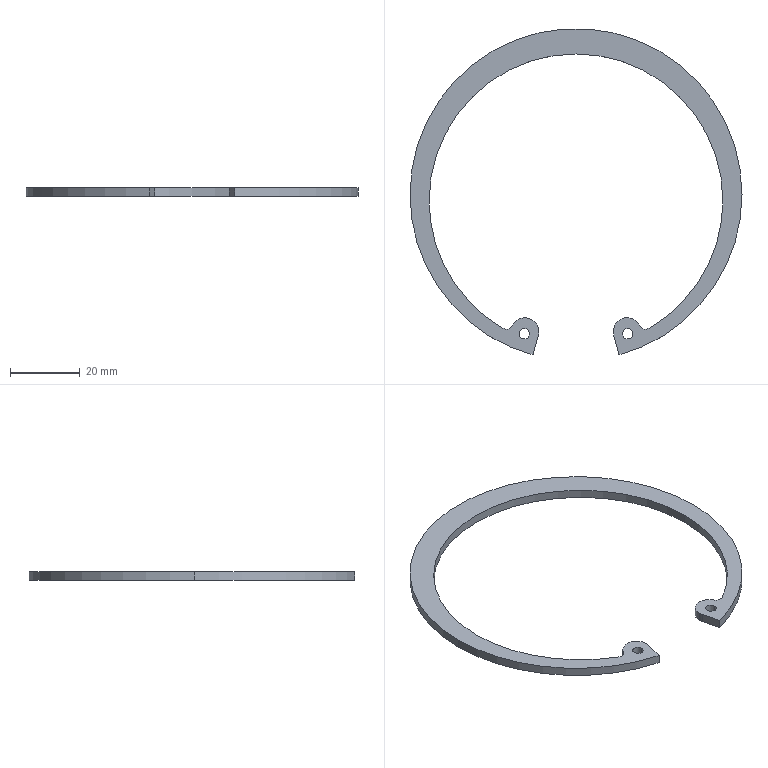Part | SolidWorks | features Extrusion 1 | 1 solid | 19 faces | box 95.5 x 93.873 x 2.5 mm | volume 3834 mm3 | cylinder 15 | plane 4 | commonest cylinder face diameters 3 x4 8 x3 84.5 x3 95.5 x3 4 x2
STEP:
#1=CARTESIAN_POINT('',(13.367,-40.028,1.25));
#2=VERTEX_POINT('',#1);
#3=CARTESIAN_POINT('',(16.367,-40.028,1.25));
#4=VERTEX_POINT('',#3);
#5=CARTESIAN_POINT('',(14.867,-40.028,1.25));
#6=DIRECTION('',(0.,0.,1.));
#7=DIRECTION('',(-1.,0.,0.));
#8=AXIS2_PLACEMENT_3D('',#5,#6,#7);
#9=CIRCLE('',#8,1.5);
#10=EDGE_CURVE('',#2,#4,#9,.T.);
#11=ORIENTED_EDGE('',*,*,#10,.T.);
#12=CARTESIAN_POINT('',(16.367,-40.028,-1.25));
#13=VERTEX_POINT('',#12);
#14=CARTESIAN_POINT('',(16.367,-40.028,1.25));
#15=DIRECTION('',(0.,0.,-1.));
#16=VECTOR('',#15,1000.);
#17=LINE('',#14,#16);
#18=EDGE_CURVE('',#4,#13,#17,.T.);
#19=ORIENTED_EDGE('',*,*,#18,.T.);
#20=CARTESIAN_POINT('',(13.367,-40.028,-1.25));
#21=VERTEX_POINT('',#20);
#22=CARTESIAN_POINT('',(14.867,-40.028,-1.25));
#23=DIRECTION('',(0.,0.,1.));
#24=DIRECTION('',(-1.,0.,0.));
#25=AXIS2_PLACEMENT_3D('',#22,#23,#24);
#26=CIRCLE('',#25,1.5);
#27=EDGE_CURVE('',#21,#13,#26,.T.);
#28=ORIENTED_EDGE('',*,*,#27,.F.);
#29=CARTESIAN_POINT('',(13.367,-40.028,1.25));
#30=DIRECTION('',(0.,0.,-1.));
#31=VECTOR('',#30,1000.);
#32=LINE('',#29,#31);
#33=EDGE_CURVE('',#2,#21,#32,.T.);
#34=ORIENTED_EDGE('',*,*,#33,.F.);
#35=EDGE_LOOP('',(#11,#19,#28,#34));
#36=FACE_OUTER_BOUND('',#35,.T.);
#37=CARTESIAN_POINT('',(14.867,-40.028,1.25));
#38=DIRECTION('',(0.,0.,-1.));
#39=DIRECTION('',(-1.,0.,0.));
#40=AXIS2_PLACEMENT_3D('',#37,#38,#39);
#41=CYLINDRICAL_SURFACE('',#40,1.5);
#42=ADVANCED_FACE('',(#36),#41,.F.);
#43=CARTESIAN_POINT('',(-16.367,-40.028,1.25));
#44=VERTEX_POINT('',#43);
#45=CARTESIAN_POINT('',(-13.367,-40.028,1.25));
#46=VERTEX_POINT('',#45);
#47=CARTESIAN_POINT('',(-14.867,-40.028,1.25));
#48=DIRECTION('',(0.,0.,1.));
#49=DIRECTION('',(1.,0.,0.));
#50=AXIS2_PLACEMENT_3D('',#47,#48,#49);
#51=CIRCLE('',#50,1.5);
#52=EDGE_CURVE('',#44,#46,#51,.T.);
#53=ORIENTED_EDGE('',*,*,#52,.T.);
#54=CARTESIAN_POINT('',(-13.367,-40.028,-1.25));
#55=VERTEX_POINT('',#54);
#56=CARTESIAN_POINT('',(-13.367,-40.028,1.25));
#57=DIRECTION('',(0.,0.,-1.));
#58=VECTOR('',#57,1000.);
#59=LINE('',#56,#58);
#60=EDGE_CURVE('',#46,#55,#59,.T.);
#61=ORIENTED_EDGE('',*,*,#60,.T.);
#62=CARTESIAN_POINT('',(-16.367,-40.028,-1.25));
#63=VERTEX_POINT('',#62);
#64=CARTESIAN_POINT('',(-14.867,-40.028,-1.25));
#65=DIRECTION('',(0.,0.,1.));
#66=DIRECTION('',(1.,0.,0.));
#67=AXIS2_PLACEMENT_3D('',#64,#65,#66);
#68=CIRCLE('',#67,1.5);
#69=EDGE_CURVE('',#63,#55,#68,.T.);
#70=ORIENTED_EDGE('',*,*,#69,.F.);
#71=CARTESIAN_POINT('',(-16.367,-40.028,1.25));
#72=DIRECTION('',(0.,0.,-1.));
#73=VECTOR('',#72,1000.);
#74=LINE('',#71,#73);
#75=EDGE_CURVE('',#44,#63,#74,.T.);
#76=ORIENTED_EDGE('',*,*,#75,.F.);
#77=EDGE_LOOP('',(#53,#61,#70,#76));
#78=FACE_OUTER_BOUND('',#77,.T.);
#79=CARTESIAN_POINT('',(-14.867,-40.028,1.25));
#80=DIRECTION('',(0.,0.,-1.));
#81=DIRECTION('',(-1.,0.,0.));
#82=AXIS2_PLACEMENT_3D('',#79,#80,#81);
#83=CYLINDRICAL_SURFACE('',#82,1.5);
#84=ADVANCED_FACE('',(#78),#83,.F.);
#85=CARTESIAN_POINT('',(47.75,0.,1.25));
#86=VERTEX_POINT('',#85);
#87=CARTESIAN_POINT('',(-47.75,0.,1.25));
#88=VERTEX_POINT('',#87);
#89=CARTESIAN_POINT('',(0.,0.,1.25));
#90=DIRECTION('',(0.,0.,1.));
#91=DIRECTION('',(1.,0.,0.));
#92=AXIS2_PLACEMENT_3D('',#89,#90,#91);
#93=CIRCLE('',#92,47.75);
#94=EDGE_CURVE('',#86,#88,#93,.T.);
#95=ORIENTED_EDGE('',*,*,#94,.F.);
#96=CARTESIAN_POINT('',(47.75,0.,-1.25));
#97=VERTEX_POINT('',#96);
#98=CARTESIAN_POINT('',(47.75,0.,1.25));
#99=DIRECTION('',(0.,0.,-1.));
#100=VECTOR('',#99,1000.);
#101=LINE('',#98,#100);
#102=EDGE_CURVE('',#86,#97,#101,.T.);
#103=ORIENTED_EDGE('',*,*,#102,.T.);
#104=CARTESIAN_POINT('',(-47.75,0.,-1.25));
#105=VERTEX_POINT('',#104);
#106=CARTESIAN_POINT('',(0.,0.,-1.25));
#107=DIRECTION('',(0.,0.,1.));
#108=DIRECTION('',(1.,0.,0.));
#109=AXIS2_PLACEMENT_3D('',#106,#107,#108);
#110=CIRCLE('',#109,47.75);
#111=EDGE_CURVE('',#97,#105,#110,.T.);
#112=ORIENTED_EDGE('',*,*,#111,.T.);
#113=CARTESIAN_POINT('',(-47.75,0.,1.25));
#114=DIRECTION('',(0.,0.,-1.));
#115=VECTOR('',#114,1000.);
#116=LINE('',#113,#115);
#117=EDGE_CURVE('',#88,#105,#116,.T.);
#118=ORIENTED_EDGE('',*,*,#117,.F.);
#119=EDGE_LOOP('',(#95,#103,#112,#118));
#120=FACE_OUTER_BOUND('',#119,.T.);
#121=CARTESIAN_POINT('',(0.,0.,1.25));
#122=DIRECTION('',(0.,0.,-1.));
#123=DIRECTION('',(-1.,0.,0.));
#124=AXIS2_PLACEMENT_3D('',#121,#122,#123);
#125=CYLINDRICAL_SURFACE('',#124,47.75);
#126=ADVANCED_FACE('',(#120),#125,.T.);
#127=CARTESIAN_POINT('',(-12.359,-46.123,1.25));
#128=VERTEX_POINT('',#127);
#129=CARTESIAN_POINT('',(0.,0.,1.25));
#130=DIRECTION('',(0.,0.,1.));
#131=DIRECTION('',(1.,0.,0.));
#132=AXIS2_PLACEMENT_3D('',#129,#130,#131);
#133=CIRCLE('',#132,47.75);
#134=EDGE_CURVE('',#88,#128,#133,.T.);
#135=ORIENTED_EDGE('',*,*,#134,.F.);
#136=ORIENTED_EDGE('',*,*,#117,.T.);
#137=CARTESIAN_POINT('',(-12.359,-46.123,-1.25));
#138=VERTEX_POINT('',#137);
#139=CARTESIAN_POINT('',(0.,0.,-1.25));
#140=DIRECTION('',(0.,0.,1.));
#141=DIRECTION('',(1.,0.,0.));
#142=AXIS2_PLACEMENT_3D('',#139,#140,#141);
#143=CIRCLE('',#142,47.75);
#144=EDGE_CURVE('',#105,#138,#143,.T.);
#145=ORIENTED_EDGE('',*,*,#144,.T.);
#146=CARTESIAN_POINT('',(-12.359,-46.123,1.25));
#147=DIRECTION('',(0.,0.,-1.));
#148=VECTOR('',#147,1000.);
#149=LINE('',#146,#148);
#150=EDGE_CURVE('',#128,#138,#149,.T.);
#151=ORIENTED_EDGE('',*,*,#150,.F.);
#152=EDGE_LOOP('',(#135,#136,#145,#151));
#153=FACE_OUTER_BOUND('',#152,.T.);
#154=CARTESIAN_POINT('',(0.,0.,1.25));
#155=DIRECTION('',(0.,0.,-1.));
#156=DIRECTION('',(-1.,0.,0.));
#157=AXIS2_PLACEMENT_3D('',#154,#155,#156);
#158=CYLINDRICAL_SURFACE('',#157,47.75);
#159=ADVANCED_FACE('',(#153),#158,.T.);
#160=CARTESIAN_POINT('',(10.698,-39.398,1.25));
#161=VERTEX_POINT('',#160);
#162=CARTESIAN_POINT('',(10.834,-40.433,1.25));
#163=VERTEX_POINT('',#162);
#164=CARTESIAN_POINT('',(14.698,-39.398,1.25));
#165=DIRECTION('',(0.,0.,1.));
#166=DIRECTION('',(-1.,0.,0.));
#167=AXIS2_PLACEMENT_3D('',#164,#165,#166);
#168=CIRCLE('',#167,4.);
#169=EDGE_CURVE('',#161,#163,#168,.T.);
#170=ORIENTED_EDGE('',*,*,#169,.F.);
#171=CARTESIAN_POINT('',(10.698,-39.398,-1.25));
#172=VERTEX_POINT('',#171);
#173=CARTESIAN_POINT('',(10.698,-39.398,1.25));
#174=DIRECTION('',(0.,0.,-1.));
#175=VECTOR('',#174,1000.);
#176=LINE('',#173,#175);
#177=EDGE_CURVE('',#161,#172,#176,.T.);
#178=ORIENTED_EDGE('',*,*,#177,.T.);
#179=CARTESIAN_POINT('',(10.834,-40.433,-1.25));
#180=VERTEX_POINT('',#179);
#181=CARTESIAN_POINT('',(14.698,-39.398,-1.25));
#182=DIRECTION('',(0.,0.,1.));
#183=DIRECTION('',(-1.,0.,0.));
#184=AXIS2_PLACEMENT_3D('',#181,#182,#183);
#185=CIRCLE('',#184,4.);
#186=EDGE_CURVE('',#172,#180,#185,.T.);
#187=ORIENTED_EDGE('',*,*,#186,.T.);
#188=CARTESIAN_POINT('',(10.834,-40.433,1.25));
#189=DIRECTION('',(0.,0.,-1.));
#190=VECTOR('',#189,1000.);
#191=LINE('',#188,#190);
#192=EDGE_CURVE('',#163,#180,#191,.T.);
#193=ORIENTED_EDGE('',*,*,#192,.F.);
#194=EDGE_LOOP('',(#170,#178,#187,#193));
#195=FACE_OUTER_BOUND('',#194,.T.);
#196=CARTESIAN_POINT('',(14.698,-39.398,1.25));
#197=DIRECTION('',(0.,0.,-1.));
#198=DIRECTION('',(-1.,0.,0.));
#199=AXIS2_PLACEMENT_3D('',#196,#197,#198);
#200=CYLINDRICAL_SURFACE('',#199,4.);
#201=ADVANCED_FACE('',(#195),#200,.T.);
#202=CARTESIAN_POINT('',(42.25,-1.8,1.25));
#203=VERTEX_POINT('',#202);
#204=CARTESIAN_POINT('',(21.052,-38.431,1.25));
#205=VERTEX_POINT('',#204);
#206=CARTESIAN_POINT('',(0.,-1.8,1.25));
#207=DIRECTION('',(0.,0.,-1.));
#208=DIRECTION('',(1.,0.,0.));
#209=AXIS2_PLACEMENT_3D('',#206,#207,#208);
#210=CIRCLE('',#209,42.25);
#211=EDGE_CURVE('',#203,#205,#210,.T.);
#212=ORIENTED_EDGE('',*,*,#211,.F.);
#213=CARTESIAN_POINT('',(42.25,-1.8,-1.25));
#214=VERTEX_POINT('',#213);
#215=CARTESIAN_POINT('',(42.25,-1.8,1.25));
#216=DIRECTION('',(0.,0.,-1.));
#217=VECTOR('',#216,1000.);
#218=LINE('',#215,#217);
#219=EDGE_CURVE('',#203,#214,#218,.T.);
#220=ORIENTED_EDGE('',*,*,#219,.T.);
#221=CARTESIAN_POINT('',(21.052,-38.431,-1.25));
#222=VERTEX_POINT('',#221);
#223=CARTESIAN_POINT('',(0.,-1.8,-1.25));
#224=DIRECTION('',(0.,0.,-1.));
#225=DIRECTION('',(1.,0.,0.));
#226=AXIS2_PLACEMENT_3D('',#223,#224,#225);
#227=CIRCLE('',#226,42.25);
#228=EDGE_CURVE('',#214,#222,#227,.T.);
#229=ORIENTED_EDGE('',*,*,#228,.T.);
#230=CARTESIAN_POINT('',(21.052,-38.431,1.25));
#231=DIRECTION('',(0.,0.,-1.));
#232=VECTOR('',#231,1000.);
#233=LINE('',#230,#232);
#234=EDGE_CURVE('',#205,#222,#233,.T.);
#235=ORIENTED_EDGE('',*,*,#234,.F.);
#236=EDGE_LOOP('',(#212,#220,#229,#235));
#237=FACE_OUTER_BOUND('',#236,.T.);
#238=CARTESIAN_POINT('',(0.,-1.8,1.25));
#239=DIRECTION('',(0.,0.,-1.));
#240=DIRECTION('',(-1.,0.,0.));
#241=AXIS2_PLACEMENT_3D('',#238,#239,#240);
#242=CYLINDRICAL_SURFACE('',#241,42.25);
#243=ADVANCED_FACE('',(#237),#242,.F.);
#244=ORIENTED_EDGE('',*,*,#219,.F.);
#245=CARTESIAN_POINT('',(-42.25,-1.8,1.25));
#246=VERTEX_POINT('',#245);
#247=CARTESIAN_POINT('',(0.,-1.8,1.25));
#248=DIRECTION('',(0.,0.,-1.));
#249=DIRECTION('',(1.,0.,0.));
#250=AXIS2_PLACEMENT_3D('',#247,#248,#249);
#251=CIRCLE('',#250,42.25);
#252=EDGE_CURVE('',#246,#203,#251,.T.);
#253=ORIENTED_EDGE('',*,*,#252,.F.);
#254=CARTESIAN_POINT('',(-42.25,-1.8,-1.25));
#255=VERTEX_POINT('',#254);
#256=CARTESIAN_POINT('',(-42.25,-1.8,1.25));
#257=DIRECTION('',(0.,0.,-1.));
#258=VECTOR('',#257,1000.);
#259=LINE('',#256,#258);
#260=EDGE_CURVE('',#246,#255,#259,.T.);
#261=ORIENTED_EDGE('',*,*,#260,.T.);
#262=CARTESIAN_POINT('',(0.,-1.8,-1.25));
#263=DIRECTION('',(0.,0.,-1.));
#264=DIRECTION('',(1.,0.,0.));
#265=AXIS2_PLACEMENT_3D('',#262,#263,#264);
#266=CIRCLE('',#265,42.25);
#267=EDGE_CURVE('',#255,#214,#266,.T.);
#268=ORIENTED_EDGE('',*,*,#267,.T.);
#269=EDGE_LOOP('',(#244,#253,#261,#268));
#270=FACE_OUTER_BOUND('',#269,.T.);
#271=CARTESIAN_POINT('',(0.,-1.8,1.25));
#272=DIRECTION('',(0.,0.,-1.));
#273=DIRECTION('',(-1.,0.,0.));
#274=AXIS2_PLACEMENT_3D('',#271,#272,#273);
#275=CYLINDRICAL_SURFACE('',#274,42.25);
#276=ADVANCED_FACE('',(#270),#275,.F.);
#277=ORIENTED_EDGE('',*,*,#52,.F.);
#278=CARTESIAN_POINT('',(-14.867,-40.028,1.25));
#279=DIRECTION('',(0.,0.,1.));
#280=DIRECTION('',(1.,0.,0.));
#281=AXIS2_PLACEMENT_3D('',#278,#279,#280);
#282=CIRCLE('',#281,1.5);
#283=EDGE_CURVE('',#46,#44,#282,.T.);
#284=ORIENTED_EDGE('',*,*,#283,.F.);
#285=EDGE_LOOP('',(#277,#284));
#286=FACE_BOUND('',#285,.T.);
#287=CARTESIAN_POINT('',(-10.834,-40.433,1.25));
#288=VERTEX_POINT('',#287);
#289=CARTESIAN_POINT('',(-18.27,-37.598,1.25));
#290=VERTEX_POINT('',#289);
#291=CARTESIAN_POINT('',(-14.698,-39.398,1.25));
#292=DIRECTION('',(0.,0.,1.));
#293=DIRECTION('',(1.,0.,0.));
#294=AXIS2_PLACEMENT_3D('',#291,#292,#293);
#295=CIRCLE('',#294,4.);
#296=EDGE_CURVE('',#288,#290,#295,.T.);
#297=ORIENTED_EDGE('',*,*,#296,.T.);
#298=CARTESIAN_POINT('',(-21.052,-38.431,1.25));
#299=VERTEX_POINT('',#298);
#300=CARTESIAN_POINT('',(-20.056,-36.697,1.25));
#301=DIRECTION('',(0.,0.,-1.));
#302=DIRECTION('',(-1.,0.,0.));
#303=AXIS2_PLACEMENT_3D('',#300,#301,#302);
#304=CIRCLE('',#303,2.);
#305=EDGE_CURVE('',#290,#299,#304,.T.);
#306=ORIENTED_EDGE('',*,*,#305,.T.);
#307=CARTESIAN_POINT('',(0.,-1.8,1.25));
#308=DIRECTION('',(0.,0.,-1.));
#309=DIRECTION('',(1.,0.,0.));
#310=AXIS2_PLACEMENT_3D('',#307,#308,#309);
#311=CIRCLE('',#310,42.25);
#312=EDGE_CURVE('',#299,#246,#311,.T.);
#313=ORIENTED_EDGE('',*,*,#312,.T.);
#314=ORIENTED_EDGE('',*,*,#252,.T.);
#315=ORIENTED_EDGE('',*,*,#211,.T.);
#316=CARTESIAN_POINT('',(18.27,-37.598,1.25));
#317=VERTEX_POINT('',#316);
#318=CARTESIAN_POINT('',(20.056,-36.697,1.25));
#319=DIRECTION('',(0.,0.,-1.));
#320=DIRECTION('',(1.,0.,0.));
#321=AXIS2_PLACEMENT_3D('',#318,#319,#320);
#322=CIRCLE('',#321,2.);
#323=EDGE_CURVE('',#205,#317,#322,.T.);
#324=ORIENTED_EDGE('',*,*,#323,.T.);
#325=CARTESIAN_POINT('',(14.698,-39.398,1.25));
#326=DIRECTION('',(0.,0.,1.));
#327=DIRECTION('',(-1.,0.,0.));
#328=AXIS2_PLACEMENT_3D('',#325,#326,#327);
#329=CIRCLE('',#328,4.);
#330=EDGE_CURVE('',#317,#161,#329,.T.);
#331=ORIENTED_EDGE('',*,*,#330,.T.);
#332=ORIENTED_EDGE('',*,*,#169,.T.);
#333=CARTESIAN_POINT('',(12.359,-46.123,1.25));
#334=VERTEX_POINT('',#333);
#335=CARTESIAN_POINT('',(10.834,-40.433,1.25));
#336=DIRECTION('',(0.2588,-0.9659,0.));
#337=VECTOR('',#336,1000.);
#338=LINE('',#335,#337);
#339=EDGE_CURVE('',#163,#334,#338,.T.);
#340=ORIENTED_EDGE('',*,*,#339,.T.);
#341=CARTESIAN_POINT('',(0.,0.,1.25));
#342=DIRECTION('',(0.,0.,1.));
#343=DIRECTION('',(1.,0.,0.));
#344=AXIS2_PLACEMENT_3D('',#341,#342,#343);
#345=CIRCLE('',#344,47.75);
#346=EDGE_CURVE('',#334,#86,#345,.T.);
#347=ORIENTED_EDGE('',*,*,#346,.T.);
#348=ORIENTED_EDGE('',*,*,#94,.T.);
#349=ORIENTED_EDGE('',*,*,#134,.T.);
#350=CARTESIAN_POINT('',(-10.834,-40.433,1.25));
#351=DIRECTION('',(0.2588,0.9659,0.));
#352=VECTOR('',#351,1000.);
#353=LINE('',#350,#352);
#354=EDGE_CURVE('',#128,#288,#353,.T.);
#355=ORIENTED_EDGE('',*,*,#354,.T.);
#356=EDGE_LOOP('',(#297,#306,#313,#314,#315,#324,#331,#332,#340,#347,#348,#349,#355));
#357=FACE_OUTER_BOUND('',#356,.T.);
#358=ORIENTED_EDGE('',*,*,#10,.F.);
#359=CARTESIAN_POINT('',(14.867,-40.028,1.25));
#360=DIRECTION('',(0.,0.,1.));
#361=DIRECTION('',(-1.,0.,0.));
#362=AXIS2_PLACEMENT_3D('',#359,#360,#361);
#363=CIRCLE('',#362,1.5);
#364=EDGE_CURVE('',#4,#2,#363,.T.);
#365=ORIENTED_EDGE('',*,*,#364,.F.);
#366=EDGE_LOOP('',(#358,#365));
#367=FACE_BOUND('',#366,.T.);
#368=CARTESIAN_POINT('',(-14.698,-39.398,1.25));
#369=DIRECTION('',(0.,0.,1.));
#370=DIRECTION('',(1.,0.,0.));
#371=AXIS2_PLACEMENT_3D('',#368,#369,#370);
#372=PLANE('',#371);
#373=ADVANCED_FACE('',(#286,#357,#367),#372,.T.);
#374=CARTESIAN_POINT('',(-10.834,-40.433,-1.25));
#375=VERTEX_POINT('',#374);
#376=CARTESIAN_POINT('',(-10.834,-40.433,1.25));
#377=DIRECTION('',(0.,0.,-1.));
#378=VECTOR('',#377,1000.);
#379=LINE('',#376,#378);
#380=EDGE_CURVE('',#288,#375,#379,.T.);
#381=ORIENTED_EDGE('',*,*,#380,.T.);
#382=CARTESIAN_POINT('',(-18.27,-37.598,-1.25));
#383=VERTEX_POINT('',#382);
#384=CARTESIAN_POINT('',(-14.698,-39.398,-1.25));
#385=DIRECTION('',(0.,0.,1.));
#386=DIRECTION('',(1.,0.,0.));
#387=AXIS2_PLACEMENT_3D('',#384,#385,#386);
#388=CIRCLE('',#387,4.);
#389=EDGE_CURVE('',#375,#383,#388,.T.);
#390=ORIENTED_EDGE('',*,*,#389,.T.);
#391=CARTESIAN_POINT('',(-18.27,-37.598,1.25));
#392=DIRECTION('',(0.,0.,-1.));
#393=VECTOR('',#392,1000.);
#394=LINE('',#391,#393);
#395=EDGE_CURVE('',#290,#383,#394,.T.);
#396=ORIENTED_EDGE('',*,*,#395,.F.);
#397=ORIENTED_EDGE('',*,*,#296,.F.);
#398=EDGE_LOOP('',(#381,#390,#396,#397));
#399=FACE_OUTER_BOUND('',#398,.T.);
#400=CARTESIAN_POINT('',(-14.698,-39.398,1.25));
#401=DIRECTION('',(0.,0.,-1.));
#402=DIRECTION('',(-1.,0.,0.));
#403=AXIS2_PLACEMENT_3D('',#400,#401,#402);
#404=CYLINDRICAL_SURFACE('',#403,4.);
#405=ADVANCED_FACE('',(#399),#404,.T.);
#406=ORIENTED_EDGE('',*,*,#395,.T.);
#407=CARTESIAN_POINT('',(-21.052,-38.431,-1.25));
#408=VERTEX_POINT('',#407);
#409=CARTESIAN_POINT('',(-20.056,-36.697,-1.25));
#410=DIRECTION('',(0.,0.,-1.));
#411=DIRECTION('',(-1.,0.,0.));
#412=AXIS2_PLACEMENT_3D('',#409,#410,#411);
#413=CIRCLE('',#412,2.);
#414=EDGE_CURVE('',#383,#408,#413,.T.);
#415=ORIENTED_EDGE('',*,*,#414,.T.);
#416=CARTESIAN_POINT('',(-21.052,-38.431,1.25));
#417=DIRECTION('',(0.,0.,-1.));
#418=VECTOR('',#417,1000.);
#419=LINE('',#416,#418);
#420=EDGE_CURVE('',#299,#408,#419,.T.);
#421=ORIENTED_EDGE('',*,*,#420,.F.);
#422=ORIENTED_EDGE('',*,*,#305,.F.);
#423=EDGE_LOOP('',(#406,#415,#421,#422));
#424=FACE_OUTER_BOUND('',#423,.T.);
#425=CARTESIAN_POINT('',(-20.056,-36.697,1.25));
#426=DIRECTION('',(0.,0.,-1.));
#427=DIRECTION('',(-1.,0.,0.));
#428=AXIS2_PLACEMENT_3D('',#425,#426,#427);
#429=CYLINDRICAL_SURFACE('',#428,2.);
#430=ADVANCED_FACE('',(#424),#429,.F.);
#431=ORIENTED_EDGE('',*,*,#260,.F.);
#432=ORIENTED_EDGE('',*,*,#312,.F.);
#433=ORIENTED_EDGE('',*,*,#420,.T.);
#434=CARTESIAN_POINT('',(0.,-1.8,-1.25));
#435=DIRECTION('',(0.,0.,-1.));
#436=DIRECTION('',(1.,0.,0.));
#437=AXIS2_PLACEMENT_3D('',#434,#435,#436);
#438=CIRCLE('',#437,42.25);
#439=EDGE_CURVE('',#408,#255,#438,.T.);
#440=ORIENTED_EDGE('',*,*,#439,.T.);
#441=EDGE_LOOP('',(#431,#432,#433,#440));
#442=FACE_OUTER_BOUND('',#441,.T.);
#443=CARTESIAN_POINT('',(0.,-1.8,1.25));
#444=DIRECTION('',(0.,0.,-1.));
#445=DIRECTION('',(-1.,0.,0.));
#446=AXIS2_PLACEMENT_3D('',#443,#444,#445);
#447=CYLINDRICAL_SURFACE('',#446,42.25);
#448=ADVANCED_FACE('',(#442),#447,.F.);
#449=ORIENTED_EDGE('',*,*,#234,.T.);
#450=CARTESIAN_POINT('',(18.27,-37.598,-1.25));
#451=VERTEX_POINT('',#450);
#452=CARTESIAN_POINT('',(20.056,-36.697,-1.25));
#453=DIRECTION('',(0.,0.,-1.));
#454=DIRECTION('',(1.,0.,0.));
#455=AXIS2_PLACEMENT_3D('',#452,#453,#454);
#456=CIRCLE('',#455,2.);
#457=EDGE_CURVE('',#222,#451,#456,.T.);
#458=ORIENTED_EDGE('',*,*,#457,.T.);
#459=CARTESIAN_POINT('',(18.27,-37.598,1.25));
#460=DIRECTION('',(0.,0.,-1.));
#461=VECTOR('',#460,1000.);
#462=LINE('',#459,#461);
#463=EDGE_CURVE('',#317,#451,#462,.T.);
#464=ORIENTED_EDGE('',*,*,#463,.F.);
#465=ORIENTED_EDGE('',*,*,#323,.F.);
#466=EDGE_LOOP('',(#449,#458,#464,#465));
#467=FACE_OUTER_BOUND('',#466,.T.);
#468=CARTESIAN_POINT('',(20.056,-36.697,1.25));
#469=DIRECTION('',(0.,0.,-1.));
#470=DIRECTION('',(-1.,0.,0.));
#471=AXIS2_PLACEMENT_3D('',#468,#469,#470);
#472=CYLINDRICAL_SURFACE('',#471,2.);
#473=ADVANCED_FACE('',(#467),#472,.F.);
#474=ORIENTED_EDGE('',*,*,#177,.F.);
#475=ORIENTED_EDGE('',*,*,#330,.F.);
#476=ORIENTED_EDGE('',*,*,#463,.T.);
#477=CARTESIAN_POINT('',(14.698,-39.398,-1.25));
#478=DIRECTION('',(0.,0.,1.));
#479=DIRECTION('',(-1.,0.,0.));
#480=AXIS2_PLACEMENT_3D('',#477,#478,#479);
#481=CIRCLE('',#480,4.);
#482=EDGE_CURVE('',#451,#172,#481,.T.);
#483=ORIENTED_EDGE('',*,*,#482,.T.);
#484=EDGE_LOOP('',(#474,#475,#476,#483));
#485=FACE_OUTER_BOUND('',#484,.T.);
#486=CARTESIAN_POINT('',(14.698,-39.398,1.25));
#487=DIRECTION('',(0.,0.,-1.));
#488=DIRECTION('',(-1.,0.,0.));
#489=AXIS2_PLACEMENT_3D('',#486,#487,#488);
#490=CYLINDRICAL_SURFACE('',#489,4.);
#491=ADVANCED_FACE('',(#485),#490,.T.);
#492=ORIENTED_EDGE('',*,*,#192,.T.);
#493=CARTESIAN_POINT('',(12.359,-46.123,-1.25));
#494=VERTEX_POINT('',#493);
#495=CARTESIAN_POINT('',(10.834,-40.433,-1.25));
#496=DIRECTION('',(0.2588,-0.9659,0.));
#497=VECTOR('',#496,1000.);
#498=LINE('',#495,#497);
#499=EDGE_CURVE('',#180,#494,#498,.T.);
#500=ORIENTED_EDGE('',*,*,#499,.T.);
#501=CARTESIAN_POINT('',(12.359,-46.123,1.25));
#502=DIRECTION('',(0.,0.,-1.));
#503=VECTOR('',#502,1000.);
#504=LINE('',#501,#503);
#505=EDGE_CURVE('',#334,#494,#504,.T.);
#506=ORIENTED_EDGE('',*,*,#505,.F.);
#507=ORIENTED_EDGE('',*,*,#339,.F.);
#508=EDGE_LOOP('',(#492,#500,#506,#507));
#509=FACE_OUTER_BOUND('',#508,.T.);
#510=CARTESIAN_POINT('',(10.834,-40.433,1.25));
#511=DIRECTION('',(0.9659,0.2588,0.));
#512=DIRECTION('',(-0.2588,0.9659,0.));
#513=AXIS2_PLACEMENT_3D('',#510,#511,#512);
#514=PLANE('',#513);
#515=ADVANCED_FACE('',(#509),#514,.F.);
#516=ORIENTED_EDGE('',*,*,#102,.F.);
#517=ORIENTED_EDGE('',*,*,#346,.F.);
#518=ORIENTED_EDGE('',*,*,#505,.T.);
#519=CARTESIAN_POINT('',(0.,0.,-1.25));
#520=DIRECTION('',(0.,0.,1.));
#521=DIRECTION('',(1.,0.,0.));
#522=AXIS2_PLACEMENT_3D('',#519,#520,#521);
#523=CIRCLE('',#522,47.75);
#524=EDGE_CURVE('',#494,#97,#523,.T.);
#525=ORIENTED_EDGE('',*,*,#524,.T.);
#526=EDGE_LOOP('',(#516,#517,#518,#525));
#527=FACE_OUTER_BOUND('',#526,.T.);
#528=CARTESIAN_POINT('',(0.,0.,1.25));
#529=DIRECTION('',(0.,0.,-1.));
#530=DIRECTION('',(-1.,0.,0.));
#531=AXIS2_PLACEMENT_3D('',#528,#529,#530);
#532=CYLINDRICAL_SURFACE('',#531,47.75);
#533=ADVANCED_FACE('',(#527),#532,.T.);
#534=ORIENTED_EDGE('',*,*,#150,.T.);
#535=CARTESIAN_POINT('',(-10.834,-40.433,-1.25));
#536=DIRECTION('',(0.2588,0.9659,0.));
#537=VECTOR('',#536,1000.);
#538=LINE('',#535,#537);
#539=EDGE_CURVE('',#138,#375,#538,.T.);
#540=ORIENTED_EDGE('',*,*,#539,.T.);
#541=ORIENTED_EDGE('',*,*,#380,.F.);
#542=ORIENTED_EDGE('',*,*,#354,.F.);
#543=EDGE_LOOP('',(#534,#540,#541,#542));
#544=FACE_OUTER_BOUND('',#543,.T.);
#545=CARTESIAN_POINT('',(-10.834,-40.433,1.25));
#546=DIRECTION('',(-0.9659,0.2588,0.));
#547=DIRECTION('',(-0.2588,-0.9659,0.));
#548=AXIS2_PLACEMENT_3D('',#545,#546,#547);
#549=PLANE('',#548);
#550=ADVANCED_FACE('',(#544),#549,.F.);
#551=ORIENTED_EDGE('',*,*,#60,.F.);
#552=ORIENTED_EDGE('',*,*,#283,.T.);
#553=ORIENTED_EDGE('',*,*,#75,.T.);
#554=CARTESIAN_POINT('',(-14.867,-40.028,-1.25));
#555=DIRECTION('',(0.,0.,1.));
#556=DIRECTION('',(1.,0.,0.));
#557=AXIS2_PLACEMENT_3D('',#554,#555,#556);
#558=CIRCLE('',#557,1.5);
#559=EDGE_CURVE('',#55,#63,#558,.T.);
#560=ORIENTED_EDGE('',*,*,#559,.F.);
#561=EDGE_LOOP('',(#551,#552,#553,#560));
#562=FACE_OUTER_BOUND('',#561,.T.);
#563=CARTESIAN_POINT('',(-14.867,-40.028,1.25));
#564=DIRECTION('',(0.,0.,-1.));
#565=DIRECTION('',(-1.,0.,0.));
#566=AXIS2_PLACEMENT_3D('',#563,#564,#565);
#567=CYLINDRICAL_SURFACE('',#566,1.5);
#568=ADVANCED_FACE('',(#562),#567,.F.);
#569=ORIENTED_EDGE('',*,*,#18,.F.);
#570=ORIENTED_EDGE('',*,*,#364,.T.);
#571=ORIENTED_EDGE('',*,*,#33,.T.);
#572=CARTESIAN_POINT('',(14.867,-40.028,-1.25));
#573=DIRECTION('',(0.,0.,1.));
#574=DIRECTION('',(-1.,0.,0.));
#575=AXIS2_PLACEMENT_3D('',#572,#573,#574);
#576=CIRCLE('',#575,1.5);
#577=EDGE_CURVE('',#13,#21,#576,.T.);
#578=ORIENTED_EDGE('',*,*,#577,.F.);
#579=EDGE_LOOP('',(#569,#570,#571,#578));
#580=FACE_OUTER_BOUND('',#579,.T.);
#581=CARTESIAN_POINT('',(14.867,-40.028,1.25));
#582=DIRECTION('',(0.,0.,-1.));
#583=DIRECTION('',(-1.,0.,0.));
#584=AXIS2_PLACEMENT_3D('',#581,#582,#583);
#585=CYLINDRICAL_SURFACE('',#584,1.5);
#586=ADVANCED_FACE('',(#580),#585,.F.);
#587=ORIENTED_EDGE('',*,*,#27,.T.);
#588=ORIENTED_EDGE('',*,*,#577,.T.);
#589=EDGE_LOOP('',(#587,#588));
#590=FACE_BOUND('',#589,.T.);
#591=ORIENTED_EDGE('',*,*,#69,.T.);
#592=ORIENTED_EDGE('',*,*,#559,.T.);
#593=EDGE_LOOP('',(#591,#592));
#594=FACE_BOUND('',#593,.T.);
#595=ORIENTED_EDGE('',*,*,#389,.F.);
#596=ORIENTED_EDGE('',*,*,#539,.F.);
#597=ORIENTED_EDGE('',*,*,#144,.F.);
#598=ORIENTED_EDGE('',*,*,#111,.F.);
#599=ORIENTED_EDGE('',*,*,#524,.F.);
#600=ORIENTED_EDGE('',*,*,#499,.F.);
#601=ORIENTED_EDGE('',*,*,#186,.F.);
#602=ORIENTED_EDGE('',*,*,#482,.F.);
#603=ORIENTED_EDGE('',*,*,#457,.F.);
#604=ORIENTED_EDGE('',*,*,#228,.F.);
#605=ORIENTED_EDGE('',*,*,#267,.F.);
#606=ORIENTED_EDGE('',*,*,#439,.F.);
#607=ORIENTED_EDGE('',*,*,#414,.F.);
#608=EDGE_LOOP('',(#595,#596,#597,#598,#599,#600,#601,#602,#603,#604,#605,#606,#607));
#609=FACE_OUTER_BOUND('',#608,.T.);
#610=CARTESIAN_POINT('',(-14.698,-39.398,-1.25));
#611=DIRECTION('',(0.,0.,1.));
#612=DIRECTION('',(1.,0.,0.));
#613=AXIS2_PLACEMENT_3D('',#610,#611,#612);
#614=PLANE('',#613);
#615=ADVANCED_FACE('',(#590,#594,#609),#614,.F.);
#616=CLOSED_SHELL('',(#42,#84,#126,#159,#201,#243,#276,#373,#405,#430,#448,#473,#491,#515,#533,#550,#568,#586,#615));
#617=MANIFOLD_SOLID_BREP('',#616);
#618=CARTESIAN_POINT('',(0.,0.,0.));
#619=DIRECTION('',(0.,0.,1.));
#620=DIRECTION('',(1.,0.,0.));
#621=AXIS2_PLACEMENT_3D('',#618,#619,#620);
#622=(LENGTH_UNIT()NAMED_UNIT(*)SI_UNIT(.MILLI.,.METRE.));
#623=UNCERTAINTY_MEASURE_WITH_UNIT(LENGTH_MEASURE(0.00001),#622,'','');
#624=(NAMED_UNIT(*)PLANE_ANGLE_UNIT()SI_UNIT($,.RADIAN.));
#625=(NAMED_UNIT(*)SI_UNIT($,.STERADIAN.)SOLID_ANGLE_UNIT());
#626=(GEOMETRIC_REPRESENTATION_CONTEXT(3)GLOBAL_UNCERTAINTY_ASSIGNED_CONTEXT((#623))GLOBAL_UNIT_ASSIGNED_CONTEXT((#622,#624,#625))REPRESENTATION_CONTEXT('',''));
#627=ADVANCED_BREP_SHAPE_REPRESENTATION('',(#617,#621),#626);